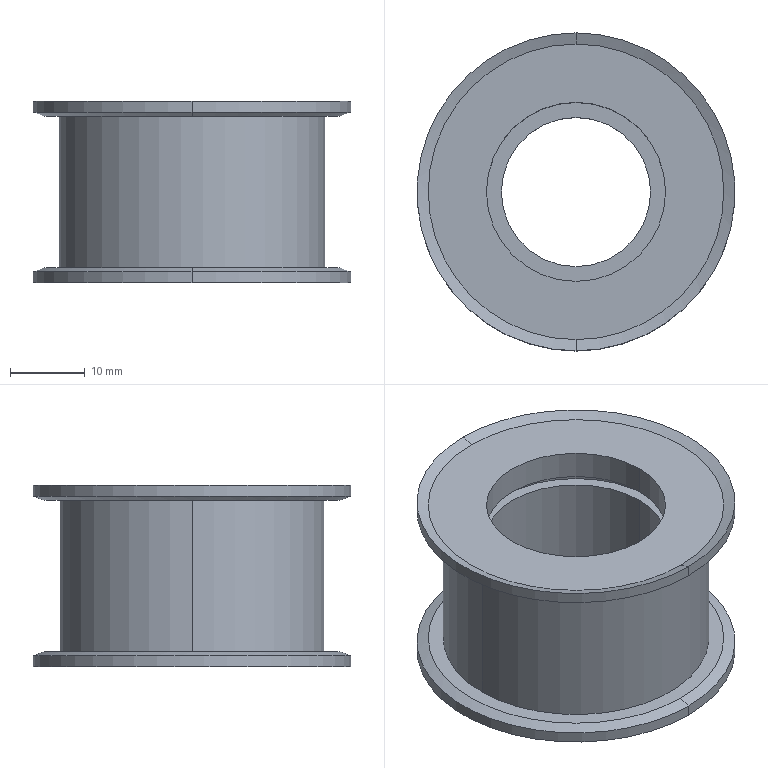Part | STEP file | Driven wheel | 1 solid | 29 faces | box 42.62 x 42.62 x 24.392 mm | volume 14671 mm3 | cylinder 14 | cone 8 | plane 7 | commonest cylinder face diameters 24 x4 42.62 x4 20 x2 27 x2 35.62 x2
STEP:
#1=CARTESIAN_POINT('',(-10.,0.,6.3));
#2=VERTEX_POINT('',#1);
#3=CARTESIAN_POINT('',(10.,0.,6.3));
#4=VERTEX_POINT('',#3);
#5=CARTESIAN_POINT('',(0.,0.,6.3));
#6=DIRECTION('',(0.,0.,1.));
#7=DIRECTION('',(1.,0.,0.));
#8=AXIS2_PLACEMENT_3D('',#5,#6,#7);
#9=CIRCLE('',#8,10.);
#10=EDGE_CURVE('',#2,#4,#9,.T.);
#11=ORIENTED_EDGE('',*,*,#10,.T.);
#12=CARTESIAN_POINT('',(10.,0.,0.));
#13=VERTEX_POINT('',#12);
#14=CARTESIAN_POINT('',(10.,0.,23.846));
#15=DIRECTION('',(0.,0.,-1.));
#16=VECTOR('',#15,1000.);
#17=LINE('',#14,#16);
#18=EDGE_CURVE('',#4,#13,#17,.T.);
#19=ORIENTED_EDGE('',*,*,#18,.T.);
#20=CARTESIAN_POINT('',(-10.,0.,0.));
#21=VERTEX_POINT('',#20);
#22=CARTESIAN_POINT('',(0.,0.,0.));
#23=DIRECTION('',(0.,0.,-1.));
#24=DIRECTION('',(-1.,0.,0.));
#25=AXIS2_PLACEMENT_3D('',#22,#23,#24);
#26=CIRCLE('',#25,10.);
#27=EDGE_CURVE('',#13,#21,#26,.T.);
#28=ORIENTED_EDGE('',*,*,#27,.T.);
#29=CARTESIAN_POINT('',(-10.,0.,23.846));
#30=DIRECTION('',(0.,0.,-1.));
#31=VECTOR('',#30,1000.);
#32=LINE('',#29,#31);
#33=EDGE_CURVE('',#2,#21,#32,.T.);
#34=ORIENTED_EDGE('',*,*,#33,.F.);
#35=EDGE_LOOP('',(#11,#19,#28,#34));
#36=FACE_OUTER_BOUND('',#35,.T.);
#37=CARTESIAN_POINT('',(0.,0.,23.846));
#38=DIRECTION('',(0.,0.,-1.));
#39=DIRECTION('',(-1.,0.,0.));
#40=AXIS2_PLACEMENT_3D('',#37,#38,#39);
#41=CYLINDRICAL_SURFACE('',#40,10.);
#42=ADVANCED_FACE('',(#36),#41,.F.);
#43=CARTESIAN_POINT('',(-12.,0.,6.3));
#44=VERTEX_POINT('',#43);
#45=CARTESIAN_POINT('',(12.,0.,6.3));
#46=VERTEX_POINT('',#45);
#47=CARTESIAN_POINT('',(0.,0.,6.3));
#48=DIRECTION('',(0.,0.,1.));
#49=DIRECTION('',(1.,0.,0.));
#50=AXIS2_PLACEMENT_3D('',#47,#48,#49);
#51=CIRCLE('',#50,12.);
#52=EDGE_CURVE('',#44,#46,#51,.T.);
#53=ORIENTED_EDGE('',*,*,#52,.F.);
#54=CARTESIAN_POINT('',(-12.,0.,18.1));
#55=VERTEX_POINT('',#54);
#56=CARTESIAN_POINT('',(-12.,0.,6.3));
#57=DIRECTION('',(0.,0.,1.));
#58=VECTOR('',#57,1000.);
#59=LINE('',#56,#58);
#60=EDGE_CURVE('',#44,#55,#59,.T.);
#61=ORIENTED_EDGE('',*,*,#60,.T.);
#62=CARTESIAN_POINT('',(12.,0.,18.1));
#63=VERTEX_POINT('',#62);
#64=CARTESIAN_POINT('',(0.,0.,18.1));
#65=DIRECTION('',(0.,0.,-1.));
#66=DIRECTION('',(1.,0.,0.));
#67=AXIS2_PLACEMENT_3D('',#64,#65,#66);
#68=CIRCLE('',#67,12.);
#69=EDGE_CURVE('',#63,#55,#68,.T.);
#70=ORIENTED_EDGE('',*,*,#69,.F.);
#71=CARTESIAN_POINT('',(12.,0.,6.3));
#72=DIRECTION('',(0.,0.,1.));
#73=VECTOR('',#72,1000.);
#74=LINE('',#71,#73);
#75=EDGE_CURVE('',#46,#63,#74,.T.);
#76=ORIENTED_EDGE('',*,*,#75,.F.);
#77=EDGE_LOOP('',(#53,#61,#70,#76));
#78=FACE_OUTER_BOUND('',#77,.T.);
#79=CARTESIAN_POINT('',(0.,0.,6.3));
#80=DIRECTION('',(0.,0.,1.));
#81=DIRECTION('',(1.,0.,0.));
#82=AXIS2_PLACEMENT_3D('',#79,#80,#81);
#83=CYLINDRICAL_SURFACE('',#82,12.);
#84=ADVANCED_FACE('',(#78),#83,.F.);
#85=CARTESIAN_POINT('',(-13.5,0.,18.1));
#86=VERTEX_POINT('',#85);
#87=CARTESIAN_POINT('',(13.5,0.,18.1));
#88=VERTEX_POINT('',#87);
#89=CARTESIAN_POINT('',(0.,0.,18.1));
#90=DIRECTION('',(0.,0.,1.));
#91=DIRECTION('',(1.,0.,0.));
#92=AXIS2_PLACEMENT_3D('',#89,#90,#91);
#93=CIRCLE('',#92,13.5);
#94=EDGE_CURVE('',#86,#88,#93,.T.);
#95=ORIENTED_EDGE('',*,*,#94,.F.);
#96=CARTESIAN_POINT('',(-13.5,0.,19.5));
#97=VERTEX_POINT('',#96);
#98=CARTESIAN_POINT('',(-13.5,0.,18.1));
#99=DIRECTION('',(0.,0.,1.));
#100=VECTOR('',#99,1000.);
#101=LINE('',#98,#100);
#102=EDGE_CURVE('',#86,#97,#101,.T.);
#103=ORIENTED_EDGE('',*,*,#102,.T.);
#104=CARTESIAN_POINT('',(13.5,0.,19.5));
#105=VERTEX_POINT('',#104);
#106=CARTESIAN_POINT('',(0.,0.,19.5));
#107=DIRECTION('',(0.,0.,1.));
#108=DIRECTION('',(1.,0.,0.));
#109=AXIS2_PLACEMENT_3D('',#106,#107,#108);
#110=CIRCLE('',#109,13.5);
#111=EDGE_CURVE('',#97,#105,#110,.T.);
#112=ORIENTED_EDGE('',*,*,#111,.T.);
#113=CARTESIAN_POINT('',(13.5,0.,18.1));
#114=DIRECTION('',(0.,0.,1.));
#115=VECTOR('',#114,1000.);
#116=LINE('',#113,#115);
#117=EDGE_CURVE('',#88,#105,#116,.T.);
#118=ORIENTED_EDGE('',*,*,#117,.F.);
#119=EDGE_LOOP('',(#95,#103,#112,#118));
#120=FACE_OUTER_BOUND('',#119,.T.);
#121=CARTESIAN_POINT('',(0.,0.,18.1));
#122=DIRECTION('',(0.,0.,1.));
#123=DIRECTION('',(1.,0.,0.));
#124=AXIS2_PLACEMENT_3D('',#121,#122,#123);
#125=CYLINDRICAL_SURFACE('',#124,13.5);
#126=ADVANCED_FACE('',(#120),#125,.F.);
#127=CARTESIAN_POINT('',(12.,0.,19.5));
#128=VERTEX_POINT('',#127);
#129=CARTESIAN_POINT('',(-12.,0.,19.5));
#130=VERTEX_POINT('',#129);
#131=CARTESIAN_POINT('',(0.,0.,19.5));
#132=DIRECTION('',(0.,0.,-1.));
#133=DIRECTION('',(1.,0.,0.));
#134=AXIS2_PLACEMENT_3D('',#131,#132,#133);
#135=CIRCLE('',#134,12.);
#136=EDGE_CURVE('',#128,#130,#135,.T.);
#137=ORIENTED_EDGE('',*,*,#136,.T.);
#138=CARTESIAN_POINT('',(-12.,0.,23.3));
#139=VERTEX_POINT('',#138);
#140=CARTESIAN_POINT('',(-12.,0.,6.3));
#141=DIRECTION('',(0.,0.,1.));
#142=VECTOR('',#141,1000.);
#143=LINE('',#140,#142);
#144=EDGE_CURVE('',#130,#139,#143,.T.);
#145=ORIENTED_EDGE('',*,*,#144,.T.);
#146=CARTESIAN_POINT('',(12.,0.,23.3));
#147=VERTEX_POINT('',#146);
#148=CARTESIAN_POINT('',(0.,0.,23.3));
#149=DIRECTION('',(0.,0.,1.));
#150=DIRECTION('',(1.,0.,0.));
#151=AXIS2_PLACEMENT_3D('',#148,#149,#150);
#152=CIRCLE('',#151,12.);
#153=EDGE_CURVE('',#139,#147,#152,.T.);
#154=ORIENTED_EDGE('',*,*,#153,.T.);
#155=CARTESIAN_POINT('',(12.,0.,6.3));
#156=DIRECTION('',(0.,0.,1.));
#157=VECTOR('',#156,1000.);
#158=LINE('',#155,#157);
#159=EDGE_CURVE('',#128,#147,#158,.T.);
#160=ORIENTED_EDGE('',*,*,#159,.F.);
#161=EDGE_LOOP('',(#137,#145,#154,#160));
#162=FACE_OUTER_BOUND('',#161,.T.);
#163=CARTESIAN_POINT('',(0.,0.,6.3));
#164=DIRECTION('',(0.,0.,1.));
#165=DIRECTION('',(1.,0.,0.));
#166=AXIS2_PLACEMENT_3D('',#163,#164,#165);
#167=CYLINDRICAL_SURFACE('',#166,12.);
#168=ADVANCED_FACE('',(#162),#167,.F.);
#169=CARTESIAN_POINT('',(0.,-19.81,1.5));
#170=VERTEX_POINT('',#169);
#171=CARTESIAN_POINT('',(0.,19.81,1.5));
#172=VERTEX_POINT('',#171);
#173=CARTESIAN_POINT('',(0.,0.,1.5));
#174=DIRECTION('',(0.,0.,1.));
#175=DIRECTION('',(0.,-1.,0.));
#176=AXIS2_PLACEMENT_3D('',#173,#174,#175);
#177=CIRCLE('',#176,19.81);
#178=EDGE_CURVE('',#170,#172,#177,.T.);
#179=ORIENTED_EDGE('',*,*,#178,.F.);
#180=CARTESIAN_POINT('',(0.,-21.31,0.954));
#181=VERTEX_POINT('',#180);
#182=CARTESIAN_POINT('',(0.,-21.31,0.954));
#183=DIRECTION('',(0.,-0.9397,-0.342));
#184=VECTOR('',#183,1000.);
#185=LINE('',#182,#184);
#186=EDGE_CURVE('',#170,#181,#185,.T.);
#187=ORIENTED_EDGE('',*,*,#186,.T.);
#188=CARTESIAN_POINT('',(0.,21.31,0.954));
#189=VERTEX_POINT('',#188);
#190=CARTESIAN_POINT('',(0.,0.,0.954));
#191=DIRECTION('',(0.,0.,1.));
#192=DIRECTION('',(0.,-1.,0.));
#193=AXIS2_PLACEMENT_3D('',#190,#191,#192);
#194=CIRCLE('',#193,21.31);
#195=EDGE_CURVE('',#181,#189,#194,.T.);
#196=ORIENTED_EDGE('',*,*,#195,.T.);
#197=CARTESIAN_POINT('',(0.,21.31,0.954));
#198=DIRECTION('',(0.,0.9397,-0.342));
#199=VECTOR('',#198,1000.);
#200=LINE('',#197,#199);
#201=EDGE_CURVE('',#172,#189,#200,.T.);
#202=ORIENTED_EDGE('',*,*,#201,.F.);
#203=EDGE_LOOP('',(#179,#187,#196,#202));
#204=FACE_OUTER_BOUND('',#203,.T.);
#205=CARTESIAN_POINT('',(0.,0.,0.954));
#206=DIRECTION('',(0.,0.,-1.));
#207=DIRECTION('',(0.,1.,0.));
#208=AXIS2_PLACEMENT_3D('',#205,#206,#207);
#209=CONICAL_SURFACE('',#208,21.31,1.222);
#210=ADVANCED_FACE('',(#204),#209,.T.);
#211=CARTESIAN_POINT('',(0.,-21.31,-0.546));
#212=VERTEX_POINT('',#211);
#213=CARTESIAN_POINT('',(0.,21.31,-0.546));
#214=VERTEX_POINT('',#213);
#215=CARTESIAN_POINT('',(0.,0.,-0.546));
#216=DIRECTION('',(0.,0.,1.));
#217=DIRECTION('',(0.,-1.,0.));
#218=AXIS2_PLACEMENT_3D('',#215,#216,#217);
#219=CIRCLE('',#218,21.31);
#220=EDGE_CURVE('',#212,#214,#219,.T.);
#221=ORIENTED_EDGE('',*,*,#220,.T.);
#222=CARTESIAN_POINT('',(0.,21.31,23.3));
#223=DIRECTION('',(0.,0.,1.));
#224=VECTOR('',#223,1000.);
#225=LINE('',#222,#224);
#226=EDGE_CURVE('',#214,#189,#225,.T.);
#227=ORIENTED_EDGE('',*,*,#226,.T.);
#228=ORIENTED_EDGE('',*,*,#195,.F.);
#229=CARTESIAN_POINT('',(0.,-21.31,23.3));
#230=DIRECTION('',(0.,0.,1.));
#231=VECTOR('',#230,1000.);
#232=LINE('',#229,#231);
#233=EDGE_CURVE('',#212,#181,#232,.T.);
#234=ORIENTED_EDGE('',*,*,#233,.F.);
#235=EDGE_LOOP('',(#221,#227,#228,#234));
#236=FACE_OUTER_BOUND('',#235,.T.);
#237=CARTESIAN_POINT('',(0.,0.,23.3));
#238=DIRECTION('',(0.,0.,1.));
#239=DIRECTION('',(0.,-1.,0.));
#240=AXIS2_PLACEMENT_3D('',#237,#238,#239);
#241=CYLINDRICAL_SURFACE('',#240,21.31);
#242=ADVANCED_FACE('',(#236),#241,.T.);
#243=CARTESIAN_POINT('',(0.,19.81,0.));
#244=VERTEX_POINT('',#243);
#245=CARTESIAN_POINT('',(0.,-19.81,0.));
#246=VERTEX_POINT('',#245);
#247=CARTESIAN_POINT('',(0.,0.,0.));
#248=DIRECTION('',(0.,0.,1.));
#249=DIRECTION('',(0.,-1.,0.));
#250=AXIS2_PLACEMENT_3D('',#247,#248,#249);
#251=CIRCLE('',#250,19.81);
#252=EDGE_CURVE('',#244,#246,#251,.T.);
#253=ORIENTED_EDGE('',*,*,#252,.T.);
#254=CARTESIAN_POINT('',(0.,-19.81,0.));
#255=DIRECTION('',(0.,-0.9397,-0.342));
#256=VECTOR('',#255,1000.);
#257=LINE('',#254,#256);
#258=EDGE_CURVE('',#246,#212,#257,.T.);
#259=ORIENTED_EDGE('',*,*,#258,.T.);
#260=CARTESIAN_POINT('',(0.,0.,-0.546));
#261=DIRECTION('',(0.,0.,1.));
#262=DIRECTION('',(0.,-1.,0.));
#263=AXIS2_PLACEMENT_3D('',#260,#261,#262);
#264=CIRCLE('',#263,21.31);
#265=EDGE_CURVE('',#214,#212,#264,.T.);
#266=ORIENTED_EDGE('',*,*,#265,.F.);
#267=CARTESIAN_POINT('',(0.,19.81,0.));
#268=DIRECTION('',(0.,0.9397,-0.342));
#269=VECTOR('',#268,1000.);
#270=LINE('',#267,#269);
#271=EDGE_CURVE('',#244,#214,#270,.T.);
#272=ORIENTED_EDGE('',*,*,#271,.F.);
#273=EDGE_LOOP('',(#253,#259,#266,#272));
#274=FACE_OUTER_BOUND('',#273,.T.);
#275=CARTESIAN_POINT('',(0.,0.,0.));
#276=DIRECTION('',(0.,0.,-1.));
#277=DIRECTION('',(0.,1.,0.));
#278=AXIS2_PLACEMENT_3D('',#275,#276,#277);
#279=CONICAL_SURFACE('',#278,19.81,1.222);
#280=ADVANCED_FACE('',(#274),#279,.F.);
#281=CARTESIAN_POINT('',(0.,19.81,23.3));
#282=VERTEX_POINT('',#281);
#283=CARTESIAN_POINT('',(0.,-19.81,23.3));
#284=VERTEX_POINT('',#283);
#285=CARTESIAN_POINT('',(0.,0.,23.3));
#286=DIRECTION('',(0.,0.,1.));
#287=DIRECTION('',(0.,-1.,0.));
#288=AXIS2_PLACEMENT_3D('',#285,#286,#287);
#289=CIRCLE('',#288,19.81);
#290=EDGE_CURVE('',#282,#284,#289,.T.);
#291=ORIENTED_EDGE('',*,*,#290,.F.);
#292=CARTESIAN_POINT('',(0.,21.31,23.846));
#293=VERTEX_POINT('',#292);
#294=CARTESIAN_POINT('',(0.,21.31,23.846));
#295=DIRECTION('',(0.,0.9397,0.342));
#296=VECTOR('',#295,1000.);
#297=LINE('',#294,#296);
#298=EDGE_CURVE('',#282,#293,#297,.T.);
#299=ORIENTED_EDGE('',*,*,#298,.T.);
#300=CARTESIAN_POINT('',(0.,-21.31,23.846));
#301=VERTEX_POINT('',#300);
#302=CARTESIAN_POINT('',(0.,0.,23.846));
#303=DIRECTION('',(0.,0.,1.));
#304=DIRECTION('',(0.,-1.,0.));
#305=AXIS2_PLACEMENT_3D('',#302,#303,#304);
#306=CIRCLE('',#305,21.31);
#307=EDGE_CURVE('',#293,#301,#306,.T.);
#308=ORIENTED_EDGE('',*,*,#307,.T.);
#309=CARTESIAN_POINT('',(0.,-21.31,23.846));
#310=DIRECTION('',(0.,-0.9397,0.342));
#311=VECTOR('',#310,1000.);
#312=LINE('',#309,#311);
#313=EDGE_CURVE('',#284,#301,#312,.T.);
#314=ORIENTED_EDGE('',*,*,#313,.F.);
#315=EDGE_LOOP('',(#291,#299,#308,#314));
#316=FACE_OUTER_BOUND('',#315,.T.);
#317=CARTESIAN_POINT('',(0.,0.,23.846));
#318=DIRECTION('',(0.,0.,1.));
#319=DIRECTION('',(0.,-1.,0.));
#320=AXIS2_PLACEMENT_3D('',#317,#318,#319);
#321=CONICAL_SURFACE('',#320,21.31,1.222);
#322=ADVANCED_FACE('',(#316),#321,.F.);
#323=CARTESIAN_POINT('',(0.,-21.31,22.346));
#324=VERTEX_POINT('',#323);
#325=CARTESIAN_POINT('',(0.,21.31,22.346));
#326=VERTEX_POINT('',#325);
#327=CARTESIAN_POINT('',(0.,0.,22.346));
#328=DIRECTION('',(0.,0.,1.));
#329=DIRECTION('',(0.,-1.,0.));
#330=AXIS2_PLACEMENT_3D('',#327,#328,#329);
#331=CIRCLE('',#330,21.31);
#332=EDGE_CURVE('',#324,#326,#331,.T.);
#333=ORIENTED_EDGE('',*,*,#332,.T.);
#334=CARTESIAN_POINT('',(0.,21.31,23.3));
#335=DIRECTION('',(0.,0.,1.));
#336=VECTOR('',#335,1000.);
#337=LINE('',#334,#336);
#338=EDGE_CURVE('',#326,#293,#337,.T.);
#339=ORIENTED_EDGE('',*,*,#338,.T.);
#340=CARTESIAN_POINT('',(0.,0.,23.846));
#341=DIRECTION('',(0.,0.,1.));
#342=DIRECTION('',(0.,-1.,0.));
#343=AXIS2_PLACEMENT_3D('',#340,#341,#342);
#344=CIRCLE('',#343,21.31);
#345=EDGE_CURVE('',#301,#293,#344,.T.);
#346=ORIENTED_EDGE('',*,*,#345,.F.);
#347=CARTESIAN_POINT('',(0.,-21.31,23.3));
#348=DIRECTION('',(0.,0.,1.));
#349=VECTOR('',#348,1000.);
#350=LINE('',#347,#349);
#351=EDGE_CURVE('',#324,#301,#350,.T.);
#352=ORIENTED_EDGE('',*,*,#351,.F.);
#353=EDGE_LOOP('',(#333,#339,#346,#352));
#354=FACE_OUTER_BOUND('',#353,.T.);
#355=CARTESIAN_POINT('',(0.,0.,23.3));
#356=DIRECTION('',(0.,0.,1.));
#357=DIRECTION('',(0.,-1.,0.));
#358=AXIS2_PLACEMENT_3D('',#355,#356,#357);
#359=CYLINDRICAL_SURFACE('',#358,21.31);
#360=ADVANCED_FACE('',(#354),#359,.T.);
#361=CARTESIAN_POINT('',(0.,-19.81,21.8));
#362=VERTEX_POINT('',#361);
#363=CARTESIAN_POINT('',(0.,19.81,21.8));
#364=VERTEX_POINT('',#363);
#365=CARTESIAN_POINT('',(0.,0.,21.8));
#366=DIRECTION('',(0.,0.,1.));
#367=DIRECTION('',(0.,-1.,0.));
#368=AXIS2_PLACEMENT_3D('',#365,#366,#367);
#369=CIRCLE('',#368,19.81);
#370=EDGE_CURVE('',#362,#364,#369,.T.);
#371=ORIENTED_EDGE('',*,*,#370,.T.);
#372=CARTESIAN_POINT('',(0.,19.81,21.8));
#373=DIRECTION('',(0.,0.9397,0.342));
#374=VECTOR('',#373,1000.);
#375=LINE('',#372,#374);
#376=EDGE_CURVE('',#364,#326,#375,.T.);
#377=ORIENTED_EDGE('',*,*,#376,.T.);
#378=ORIENTED_EDGE('',*,*,#332,.F.);
#379=CARTESIAN_POINT('',(0.,-19.81,21.8));
#380=DIRECTION('',(0.,-0.9397,0.342));
#381=VECTOR('',#380,1000.);
#382=LINE('',#379,#381);
#383=EDGE_CURVE('',#362,#324,#382,.T.);
#384=ORIENTED_EDGE('',*,*,#383,.F.);
#385=EDGE_LOOP('',(#371,#377,#378,#384));
#386=FACE_OUTER_BOUND('',#385,.T.);
#387=CARTESIAN_POINT('',(0.,0.,21.8));
#388=DIRECTION('',(0.,0.,1.));
#389=DIRECTION('',(0.,-1.,0.));
#390=AXIS2_PLACEMENT_3D('',#387,#388,#389);
#391=CONICAL_SURFACE('',#390,19.81,1.222);
#392=ADVANCED_FACE('',(#386),#391,.T.);
#393=CARTESIAN_POINT('',(17.81,0.,21.8));
#394=VERTEX_POINT('',#393);
#395=CARTESIAN_POINT('',(-17.81,0.,21.8));
#396=VERTEX_POINT('',#395);
#397=CARTESIAN_POINT('',(0.,0.,21.8));
#398=DIRECTION('',(0.,0.,1.));
#399=DIRECTION('',(0.,-1.,0.));
#400=AXIS2_PLACEMENT_3D('',#397,#398,#399);
#401=CIRCLE('',#400,17.81);
#402=EDGE_CURVE('',#394,#396,#401,.T.);
#403=ORIENTED_EDGE('',*,*,#402,.F.);
#404=CARTESIAN_POINT('',(17.81,0.,1.5));
#405=VERTEX_POINT('',#404);
#406=CARTESIAN_POINT('',(17.81,0.,23.3));
#407=DIRECTION('',(0.,0.,-1.));
#408=VECTOR('',#407,1000.);
#409=LINE('',#406,#408);
#410=EDGE_CURVE('',#394,#405,#409,.T.);
#411=ORIENTED_EDGE('',*,*,#410,.T.);
#412=CARTESIAN_POINT('',(-17.81,0.,1.5));
#413=VERTEX_POINT('',#412);
#414=CARTESIAN_POINT('',(0.,0.,1.5));
#415=DIRECTION('',(0.,0.,-1.));
#416=DIRECTION('',(0.,1.,0.));
#417=AXIS2_PLACEMENT_3D('',#414,#415,#416);
#418=CIRCLE('',#417,17.81);
#419=EDGE_CURVE('',#413,#405,#418,.T.);
#420=ORIENTED_EDGE('',*,*,#419,.F.);
#421=CARTESIAN_POINT('',(-17.81,0.,23.3));
#422=DIRECTION('',(0.,0.,-1.));
#423=VECTOR('',#422,1000.);
#424=LINE('',#421,#423);
#425=EDGE_CURVE('',#396,#413,#424,.T.);
#426=ORIENTED_EDGE('',*,*,#425,.F.);
#427=EDGE_LOOP('',(#403,#411,#420,#426));
#428=FACE_OUTER_BOUND('',#427,.T.);
#429=CARTESIAN_POINT('',(0.,0.,23.3));
#430=DIRECTION('',(0.,0.,-1.));
#431=DIRECTION('',(-1.,0.,0.));
#432=AXIS2_PLACEMENT_3D('',#429,#430,#431);
#433=CYLINDRICAL_SURFACE('',#432,17.81);
#434=ADVANCED_FACE('',(#428),#433,.T.);
#435=ORIENTED_EDGE('',*,*,#410,.F.);
#436=CARTESIAN_POINT('',(0.,0.,21.8));
#437=DIRECTION('',(0.,0.,1.));
#438=DIRECTION('',(0.,-1.,0.));
#439=AXIS2_PLACEMENT_3D('',#436,#437,#438);
#440=CIRCLE('',#439,17.81);
#441=EDGE_CURVE('',#396,#394,#440,.T.);
#442=ORIENTED_EDGE('',*,*,#441,.F.);
#443=ORIENTED_EDGE('',*,*,#425,.T.);
#444=CARTESIAN_POINT('',(0.,0.,1.5));
#445=DIRECTION('',(0.,0.,-1.));
#446=DIRECTION('',(0.,1.,0.));
#447=AXIS2_PLACEMENT_3D('',#444,#445,#446);
#448=CIRCLE('',#447,17.81);
#449=EDGE_CURVE('',#405,#413,#448,.T.);
#450=ORIENTED_EDGE('',*,*,#449,.F.);
#451=EDGE_LOOP('',(#435,#442,#443,#450));
#452=FACE_OUTER_BOUND('',#451,.T.);
#453=CARTESIAN_POINT('',(0.,0.,23.3));
#454=DIRECTION('',(0.,0.,-1.));
#455=DIRECTION('',(-1.,0.,0.));
#456=AXIS2_PLACEMENT_3D('',#453,#454,#455);
#457=CYLINDRICAL_SURFACE('',#456,17.81);
#458=ADVANCED_FACE('',(#452),#457,.T.);
#459=ORIENTED_EDGE('',*,*,#370,.F.);
#460=CARTESIAN_POINT('',(0.,0.,21.8));
#461=DIRECTION('',(0.,0.,1.));
#462=DIRECTION('',(0.,-1.,0.));
#463=AXIS2_PLACEMENT_3D('',#460,#461,#462);
#464=CIRCLE('',#463,19.81);
#465=EDGE_CURVE('',#364,#362,#464,.T.);
#466=ORIENTED_EDGE('',*,*,#465,.F.);
#467=EDGE_LOOP('',(#459,#466));
#468=FACE_OUTER_BOUND('',#467,.T.);
#469=ORIENTED_EDGE('',*,*,#441,.T.);
#470=ORIENTED_EDGE('',*,*,#402,.T.);
#471=EDGE_LOOP('',(#469,#470));
#472=FACE_BOUND('',#471,.T.);
#473=CARTESIAN_POINT('',(0.,17.81,21.8));
#474=DIRECTION('',(0.,0.,1.));
#475=DIRECTION('',(0.,-1.,0.));
#476=AXIS2_PLACEMENT_3D('',#473,#474,#475);
#477=PLANE('',#476);
#478=ADVANCED_FACE('',(#468,#472),#477,.F.);
#479=ORIENTED_EDGE('',*,*,#376,.F.);
#480=ORIENTED_EDGE('',*,*,#465,.T.);
#481=ORIENTED_EDGE('',*,*,#383,.T.);
#482=CARTESIAN_POINT('',(0.,0.,22.346));
#483=DIRECTION('',(0.,0.,1.));
#484=DIRECTION('',(0.,-1.,0.));
#485=AXIS2_PLACEMENT_3D('',#482,#483,#484);
#486=CIRCLE('',#485,21.31);
#487=EDGE_CURVE('',#326,#324,#486,.T.);
#488=ORIENTED_EDGE('',*,*,#487,.F.);
#489=EDGE_LOOP('',(#479,#480,#481,#488));
#490=FACE_OUTER_BOUND('',#489,.T.);
#491=CARTESIAN_POINT('',(0.,0.,21.8));
#492=DIRECTION('',(0.,0.,1.));
#493=DIRECTION('',(0.,-1.,0.));
#494=AXIS2_PLACEMENT_3D('',#491,#492,#493);
#495=CONICAL_SURFACE('',#494,19.81,1.222);
#496=ADVANCED_FACE('',(#490),#495,.T.);
#497=ORIENTED_EDGE('',*,*,#338,.F.);
#498=ORIENTED_EDGE('',*,*,#487,.T.);
#499=ORIENTED_EDGE('',*,*,#351,.T.);
#500=ORIENTED_EDGE('',*,*,#307,.F.);
#501=EDGE_LOOP('',(#497,#498,#499,#500));
#502=FACE_OUTER_BOUND('',#501,.T.);
#503=CARTESIAN_POINT('',(0.,0.,23.3));
#504=DIRECTION('',(0.,0.,1.));
#505=DIRECTION('',(0.,-1.,0.));
#506=AXIS2_PLACEMENT_3D('',#503,#504,#505);
#507=CYLINDRICAL_SURFACE('',#506,21.31);
#508=ADVANCED_FACE('',(#502),#507,.T.);
#509=ORIENTED_EDGE('',*,*,#298,.F.);
#510=CARTESIAN_POINT('',(0.,0.,23.3));
#511=DIRECTION('',(0.,0.,1.));
#512=DIRECTION('',(0.,-1.,0.));
#513=AXIS2_PLACEMENT_3D('',#510,#511,#512);
#514=CIRCLE('',#513,19.81);
#515=EDGE_CURVE('',#284,#282,#514,.T.);
#516=ORIENTED_EDGE('',*,*,#515,.F.);
#517=ORIENTED_EDGE('',*,*,#313,.T.);
#518=ORIENTED_EDGE('',*,*,#345,.T.);
#519=EDGE_LOOP('',(#509,#516,#517,#518));
#520=FACE_OUTER_BOUND('',#519,.T.);
#521=CARTESIAN_POINT('',(0.,0.,23.846));
#522=DIRECTION('',(0.,0.,1.));
#523=DIRECTION('',(0.,-1.,0.));
#524=AXIS2_PLACEMENT_3D('',#521,#522,#523);
#525=CONICAL_SURFACE('',#524,21.31,1.222);
#526=ADVANCED_FACE('',(#520),#525,.F.);
#527=CARTESIAN_POINT('',(0.,0.,23.3));
#528=DIRECTION('',(0.,0.,1.));
#529=DIRECTION('',(1.,0.,0.));
#530=AXIS2_PLACEMENT_3D('',#527,#528,#529);
#531=CIRCLE('',#530,12.);
#532=EDGE_CURVE('',#147,#139,#531,.T.);
#533=ORIENTED_EDGE('',*,*,#532,.F.);
#534=ORIENTED_EDGE('',*,*,#153,.F.);
#535=EDGE_LOOP('',(#533,#534));
#536=FACE_BOUND('',#535,.T.);
#537=ORIENTED_EDGE('',*,*,#515,.T.);
#538=ORIENTED_EDGE('',*,*,#290,.T.);
#539=EDGE_LOOP('',(#537,#538));
#540=FACE_OUTER_BOUND('',#539,.T.);
#541=CARTESIAN_POINT('',(0.,0.,23.3));
#542=DIRECTION('',(0.,0.,1.));
#543=DIRECTION('',(1.,0.,0.));
#544=AXIS2_PLACEMENT_3D('',#541,#542,#543);
#545=PLANE('',#544);
#546=ADVANCED_FACE('',(#536,#540),#545,.T.);
#547=ORIENTED_EDGE('',*,*,#419,.T.);
#548=ORIENTED_EDGE('',*,*,#449,.T.);
#549=EDGE_LOOP('',(#547,#548));
#550=FACE_BOUND('',#549,.T.);
#551=CARTESIAN_POINT('',(0.,0.,1.5));
#552=DIRECTION('',(0.,0.,1.));
#553=DIRECTION('',(0.,-1.,0.));
#554=AXIS2_PLACEMENT_3D('',#551,#552,#553);
#555=CIRCLE('',#554,19.81);
#556=EDGE_CURVE('',#172,#170,#555,.T.);
#557=ORIENTED_EDGE('',*,*,#556,.T.);
#558=ORIENTED_EDGE('',*,*,#178,.T.);
#559=EDGE_LOOP('',(#557,#558));
#560=FACE_OUTER_BOUND('',#559,.T.);
#561=CARTESIAN_POINT('',(0.,17.81,1.5));
#562=DIRECTION('',(0.,0.,-1.));
#563=DIRECTION('',(0.,1.,0.));
#564=AXIS2_PLACEMENT_3D('',#561,#562,#563);
#565=PLANE('',#564);
#566=ADVANCED_FACE('',(#550,#560),#565,.F.);
#567=ORIENTED_EDGE('',*,*,#258,.F.);
#568=CARTESIAN_POINT('',(0.,0.,0.));
#569=DIRECTION('',(0.,0.,1.));
#570=DIRECTION('',(0.,-1.,0.));
#571=AXIS2_PLACEMENT_3D('',#568,#569,#570);
#572=CIRCLE('',#571,19.81);
#573=EDGE_CURVE('',#246,#244,#572,.T.);
#574=ORIENTED_EDGE('',*,*,#573,.T.);
#575=ORIENTED_EDGE('',*,*,#271,.T.);
#576=ORIENTED_EDGE('',*,*,#220,.F.);
#577=EDGE_LOOP('',(#567,#574,#575,#576));
#578=FACE_OUTER_BOUND('',#577,.T.);
#579=CARTESIAN_POINT('',(0.,0.,0.));
#580=DIRECTION('',(0.,0.,-1.));
#581=DIRECTION('',(0.,1.,0.));
#582=AXIS2_PLACEMENT_3D('',#579,#580,#581);
#583=CONICAL_SURFACE('',#582,19.81,1.222);
#584=ADVANCED_FACE('',(#578),#583,.F.);
#585=ORIENTED_EDGE('',*,*,#226,.F.);
#586=ORIENTED_EDGE('',*,*,#265,.T.);
#587=ORIENTED_EDGE('',*,*,#233,.T.);
#588=CARTESIAN_POINT('',(0.,0.,0.954));
#589=DIRECTION('',(0.,0.,1.));
#590=DIRECTION('',(0.,-1.,0.));
#591=AXIS2_PLACEMENT_3D('',#588,#589,#590);
#592=CIRCLE('',#591,21.31);
#593=EDGE_CURVE('',#189,#181,#592,.T.);
#594=ORIENTED_EDGE('',*,*,#593,.F.);
#595=EDGE_LOOP('',(#585,#586,#587,#594));
#596=FACE_OUTER_BOUND('',#595,.T.);
#597=CARTESIAN_POINT('',(0.,0.,23.3));
#598=DIRECTION('',(0.,0.,1.));
#599=DIRECTION('',(0.,-1.,0.));
#600=AXIS2_PLACEMENT_3D('',#597,#598,#599);
#601=CYLINDRICAL_SURFACE('',#600,21.31);
#602=ADVANCED_FACE('',(#596),#601,.T.);
#603=ORIENTED_EDGE('',*,*,#186,.F.);
#604=ORIENTED_EDGE('',*,*,#556,.F.);
#605=ORIENTED_EDGE('',*,*,#201,.T.);
#606=ORIENTED_EDGE('',*,*,#593,.T.);
#607=EDGE_LOOP('',(#603,#604,#605,#606));
#608=FACE_OUTER_BOUND('',#607,.T.);
#609=CARTESIAN_POINT('',(0.,0.,0.954));
#610=DIRECTION('',(0.,0.,-1.));
#611=DIRECTION('',(0.,1.,0.));
#612=AXIS2_PLACEMENT_3D('',#609,#610,#611);
#613=CONICAL_SURFACE('',#612,21.31,1.222);
#614=ADVANCED_FACE('',(#608),#613,.T.);
#615=CARTESIAN_POINT('',(0.,0.,0.));
#616=DIRECTION('',(0.,0.,-1.));
#617=DIRECTION('',(-1.,0.,0.));
#618=AXIS2_PLACEMENT_3D('',#615,#616,#617);
#619=CIRCLE('',#618,10.);
#620=EDGE_CURVE('',#21,#13,#619,.T.);
#621=ORIENTED_EDGE('',*,*,#620,.F.);
#622=ORIENTED_EDGE('',*,*,#27,.F.);
#623=EDGE_LOOP('',(#621,#622));
#624=FACE_BOUND('',#623,.T.);
#625=ORIENTED_EDGE('',*,*,#252,.F.);
#626=ORIENTED_EDGE('',*,*,#573,.F.);
#627=EDGE_LOOP('',(#625,#626));
#628=FACE_OUTER_BOUND('',#627,.T.);
#629=CARTESIAN_POINT('',(0.,0.,0.));
#630=DIRECTION('',(0.,0.,1.));
#631=DIRECTION('',(1.,0.,0.));
#632=AXIS2_PLACEMENT_3D('',#629,#630,#631);
#633=PLANE('',#632);
#634=ADVANCED_FACE('',(#624,#628),#633,.F.);
#635=ORIENTED_EDGE('',*,*,#144,.F.);
#636=CARTESIAN_POINT('',(0.,0.,19.5));
#637=DIRECTION('',(0.,0.,-1.));
#638=DIRECTION('',(1.,0.,0.));
#639=AXIS2_PLACEMENT_3D('',#636,#637,#638);
#640=CIRCLE('',#639,12.);
#641=EDGE_CURVE('',#130,#128,#640,.T.);
#642=ORIENTED_EDGE('',*,*,#641,.T.);
#643=ORIENTED_EDGE('',*,*,#159,.T.);
#644=ORIENTED_EDGE('',*,*,#532,.T.);
#645=EDGE_LOOP('',(#635,#642,#643,#644));
#646=FACE_OUTER_BOUND('',#645,.T.);
#647=CARTESIAN_POINT('',(0.,0.,6.3));
#648=DIRECTION('',(0.,0.,1.));
#649=DIRECTION('',(1.,0.,0.));
#650=AXIS2_PLACEMENT_3D('',#647,#648,#649);
#651=CYLINDRICAL_SURFACE('',#650,12.);
#652=ADVANCED_FACE('',(#646),#651,.F.);
#653=CARTESIAN_POINT('',(0.,0.,18.1));
#654=DIRECTION('',(0.,0.,1.));
#655=DIRECTION('',(1.,0.,0.));
#656=AXIS2_PLACEMENT_3D('',#653,#654,#655);
#657=CIRCLE('',#656,13.5);
#658=EDGE_CURVE('',#88,#86,#657,.T.);
#659=ORIENTED_EDGE('',*,*,#658,.T.);
#660=ORIENTED_EDGE('',*,*,#94,.T.);
#661=EDGE_LOOP('',(#659,#660));
#662=FACE_OUTER_BOUND('',#661,.T.);
#663=ORIENTED_EDGE('',*,*,#69,.T.);
#664=CARTESIAN_POINT('',(0.,0.,18.1));
#665=DIRECTION('',(0.,0.,-1.));
#666=DIRECTION('',(1.,0.,0.));
#667=AXIS2_PLACEMENT_3D('',#664,#665,#666);
#668=CIRCLE('',#667,12.);
#669=EDGE_CURVE('',#55,#63,#668,.T.);
#670=ORIENTED_EDGE('',*,*,#669,.T.);
#671=EDGE_LOOP('',(#663,#670));
#672=FACE_BOUND('',#671,.T.);
#673=CARTESIAN_POINT('',(0.,0.,18.1));
#674=DIRECTION('',(0.,0.,1.));
#675=DIRECTION('',(1.,0.,0.));
#676=AXIS2_PLACEMENT_3D('',#673,#674,#675);
#677=PLANE('',#676);
#678=ADVANCED_FACE('',(#662,#672),#677,.T.);
#679=CARTESIAN_POINT('',(0.,0.,19.5));
#680=DIRECTION('',(0.,0.,1.));
#681=DIRECTION('',(1.,0.,0.));
#682=AXIS2_PLACEMENT_3D('',#679,#680,#681);
#683=CIRCLE('',#682,13.5);
#684=EDGE_CURVE('',#105,#97,#683,.T.);
#685=ORIENTED_EDGE('',*,*,#684,.F.);
#686=ORIENTED_EDGE('',*,*,#111,.F.);
#687=EDGE_LOOP('',(#685,#686));
#688=FACE_OUTER_BOUND('',#687,.T.);
#689=ORIENTED_EDGE('',*,*,#136,.F.);
#690=ORIENTED_EDGE('',*,*,#641,.F.);
#691=EDGE_LOOP('',(#689,#690));
#692=FACE_BOUND('',#691,.T.);
#693=CARTESIAN_POINT('',(0.,0.,19.5));
#694=DIRECTION('',(0.,0.,1.));
#695=DIRECTION('',(1.,0.,0.));
#696=AXIS2_PLACEMENT_3D('',#693,#694,#695);
#697=PLANE('',#696);
#698=ADVANCED_FACE('',(#688,#692),#697,.F.);
#699=ORIENTED_EDGE('',*,*,#102,.F.);
#700=ORIENTED_EDGE('',*,*,#658,.F.);
#701=ORIENTED_EDGE('',*,*,#117,.T.);
#702=ORIENTED_EDGE('',*,*,#684,.T.);
#703=EDGE_LOOP('',(#699,#700,#701,#702));
#704=FACE_OUTER_BOUND('',#703,.T.);
#705=CARTESIAN_POINT('',(0.,0.,18.1));
#706=DIRECTION('',(0.,0.,1.));
#707=DIRECTION('',(1.,0.,0.));
#708=AXIS2_PLACEMENT_3D('',#705,#706,#707);
#709=CYLINDRICAL_SURFACE('',#708,13.5);
#710=ADVANCED_FACE('',(#704),#709,.F.);
#711=ORIENTED_EDGE('',*,*,#10,.F.);
#712=CARTESIAN_POINT('',(0.,0.,6.3));
#713=DIRECTION('',(0.,0.,1.));
#714=DIRECTION('',(1.,0.,0.));
#715=AXIS2_PLACEMENT_3D('',#712,#713,#714);
#716=CIRCLE('',#715,10.);
#717=EDGE_CURVE('',#4,#2,#716,.T.);
#718=ORIENTED_EDGE('',*,*,#717,.F.);
#719=EDGE_LOOP('',(#711,#718));
#720=FACE_BOUND('',#719,.T.);
#721=CARTESIAN_POINT('',(0.,0.,6.3));
#722=DIRECTION('',(0.,0.,1.));
#723=DIRECTION('',(1.,0.,0.));
#724=AXIS2_PLACEMENT_3D('',#721,#722,#723);
#725=CIRCLE('',#724,12.);
#726=EDGE_CURVE('',#46,#44,#725,.T.);
#727=ORIENTED_EDGE('',*,*,#726,.T.);
#728=ORIENTED_EDGE('',*,*,#52,.T.);
#729=EDGE_LOOP('',(#727,#728));
#730=FACE_OUTER_BOUND('',#729,.T.);
#731=CARTESIAN_POINT('',(0.,0.,6.3));
#732=DIRECTION('',(0.,0.,1.));
#733=DIRECTION('',(1.,0.,0.));
#734=AXIS2_PLACEMENT_3D('',#731,#732,#733);
#735=PLANE('',#734);
#736=ADVANCED_FACE('',(#720,#730),#735,.T.);
#737=ORIENTED_EDGE('',*,*,#60,.F.);
#738=ORIENTED_EDGE('',*,*,#726,.F.);
#739=ORIENTED_EDGE('',*,*,#75,.T.);
#740=ORIENTED_EDGE('',*,*,#669,.F.);
#741=EDGE_LOOP('',(#737,#738,#739,#740));
#742=FACE_OUTER_BOUND('',#741,.T.);
#743=CARTESIAN_POINT('',(0.,0.,6.3));
#744=DIRECTION('',(0.,0.,1.));
#745=DIRECTION('',(1.,0.,0.));
#746=AXIS2_PLACEMENT_3D('',#743,#744,#745);
#747=CYLINDRICAL_SURFACE('',#746,12.);
#748=ADVANCED_FACE('',(#742),#747,.F.);
#749=ORIENTED_EDGE('',*,*,#18,.F.);
#750=ORIENTED_EDGE('',*,*,#717,.T.);
#751=ORIENTED_EDGE('',*,*,#33,.T.);
#752=ORIENTED_EDGE('',*,*,#620,.T.);
#753=EDGE_LOOP('',(#749,#750,#751,#752));
#754=FACE_OUTER_BOUND('',#753,.T.);
#755=CARTESIAN_POINT('',(0.,0.,23.846));
#756=DIRECTION('',(0.,0.,-1.));
#757=DIRECTION('',(-1.,0.,0.));
#758=AXIS2_PLACEMENT_3D('',#755,#756,#757);
#759=CYLINDRICAL_SURFACE('',#758,10.);
#760=ADVANCED_FACE('',(#754),#759,.F.);
#761=CLOSED_SHELL('',(#42,#84,#126,#168,#210,#242,#280,#322,#360,#392,#434,#458,#478,#496,#508,#526,#546,#566,#584,#602,#614,#634,#652,#678,#698,#710,#736,#748,#760));
#762=MANIFOLD_SOLID_BREP('',#761);
#763=CARTESIAN_POINT('',(0.,0.,0.));
#764=DIRECTION('',(0.,0.,1.));
#765=DIRECTION('',(1.,0.,0.));
#766=AXIS2_PLACEMENT_3D('',#763,#764,#765);
#767=(LENGTH_UNIT()NAMED_UNIT(*)SI_UNIT(.MILLI.,.METRE.));
#768=UNCERTAINTY_MEASURE_WITH_UNIT(LENGTH_MEASURE(0.00001),#767,'','');
#769=(NAMED_UNIT(*)PLANE_ANGLE_UNIT()SI_UNIT($,.RADIAN.));
#770=(NAMED_UNIT(*)SI_UNIT($,.STERADIAN.)SOLID_ANGLE_UNIT());
#771=(GEOMETRIC_REPRESENTATION_CONTEXT(3)GLOBAL_UNCERTAINTY_ASSIGNED_CONTEXT((#768))GLOBAL_UNIT_ASSIGNED_CONTEXT((#767,#769,#770))REPRESENTATION_CONTEXT('',''));
#772=ADVANCED_BREP_SHAPE_REPRESENTATION('',(#762,#766),#771);